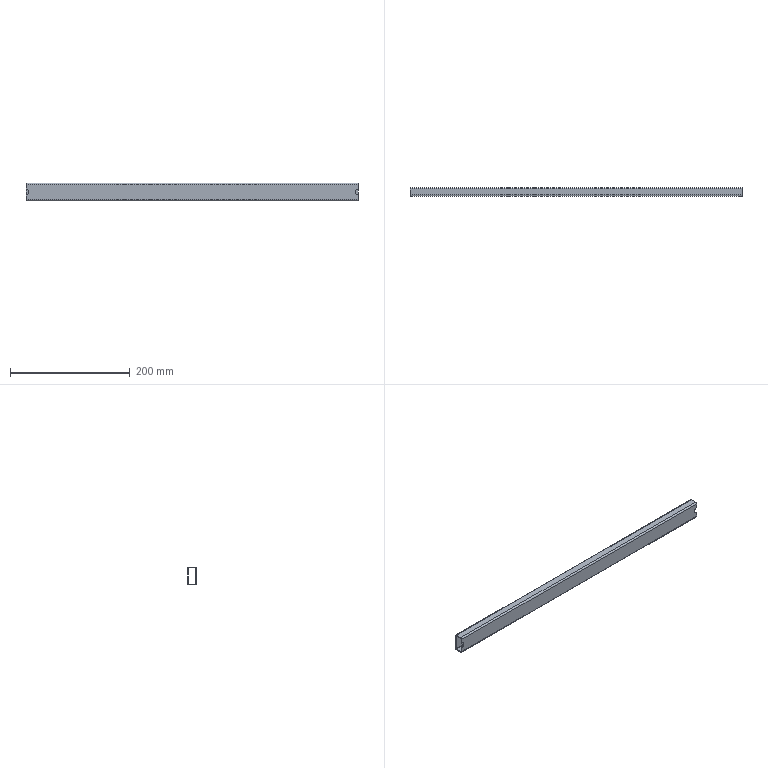Part | STEP file | 6100504 | 1 solid | 20 faces | box 555 x 15 x 30 mm | volume 67311 mm3 | plane 10 | cylinder 10 | commonest cylinder face diameters 2 x4 5 x4 10 x2